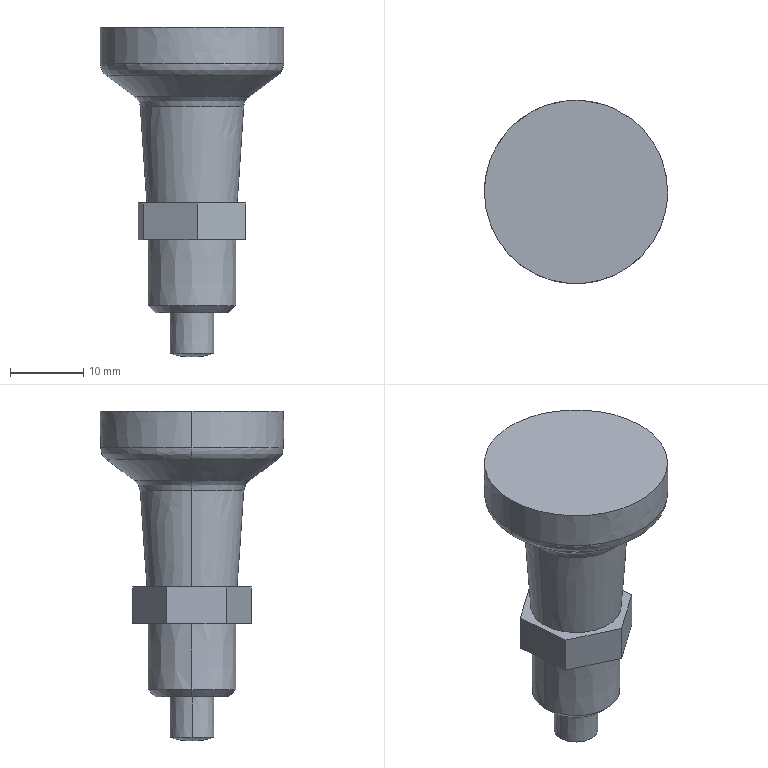Part | CATIA | 1 solid | 30 faces | box 25 x 25 x 45 mm | volume 8256 mm3 | spline 20 | plane 10